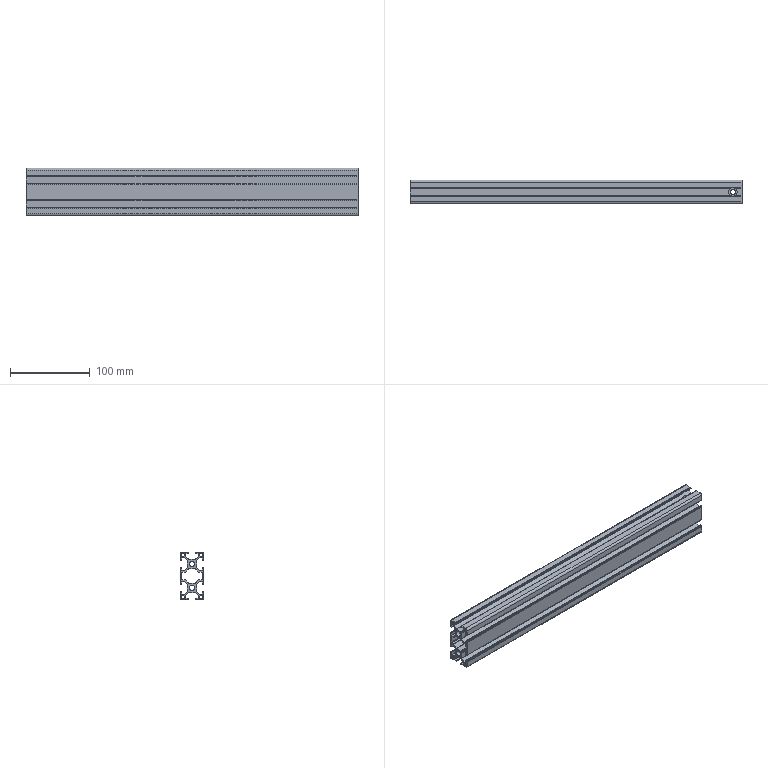Part | STEP file | 1 solid | 282 faces | box 417 x 30 x 60.001 mm | volume 241330 mm3 | cylinder 150 | plane 128 | cone 4 | commonest cylinder face diameters 0.6 x94 2 x32 6.8 x6 11 x6 5 x4 6.6 x4